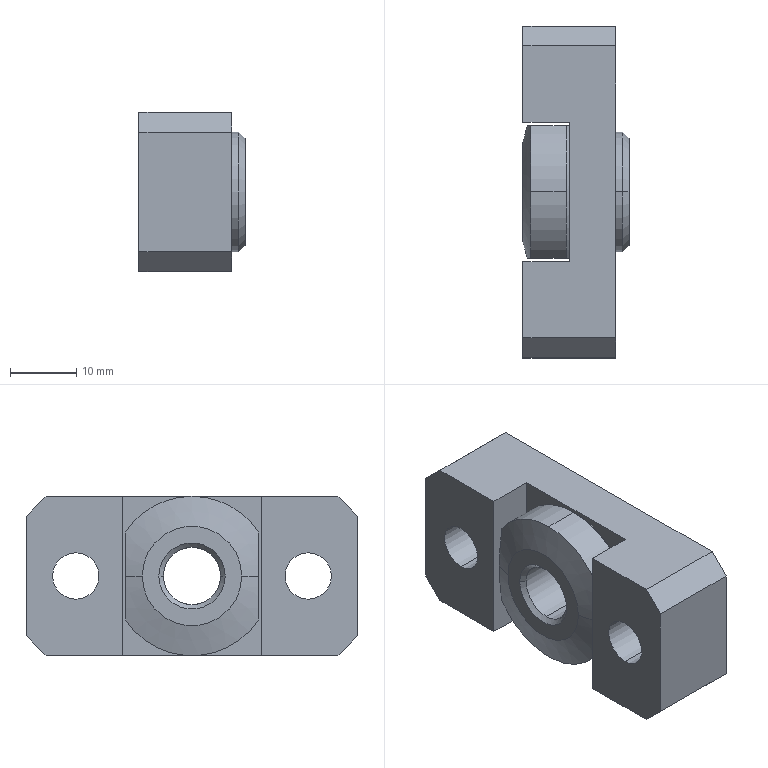Part | SolidWorks | features BaseBody 2 | 2 solids | 50 faces | box 16 x 50 x 24 mm | volume 13355 mm3 | plane 21 | cylinder 17 | cone 10 | spline 2 | commonest cylinder face diameters 7 x4 11 x4 24 x3 8.647 x2 18 x2 19 x2